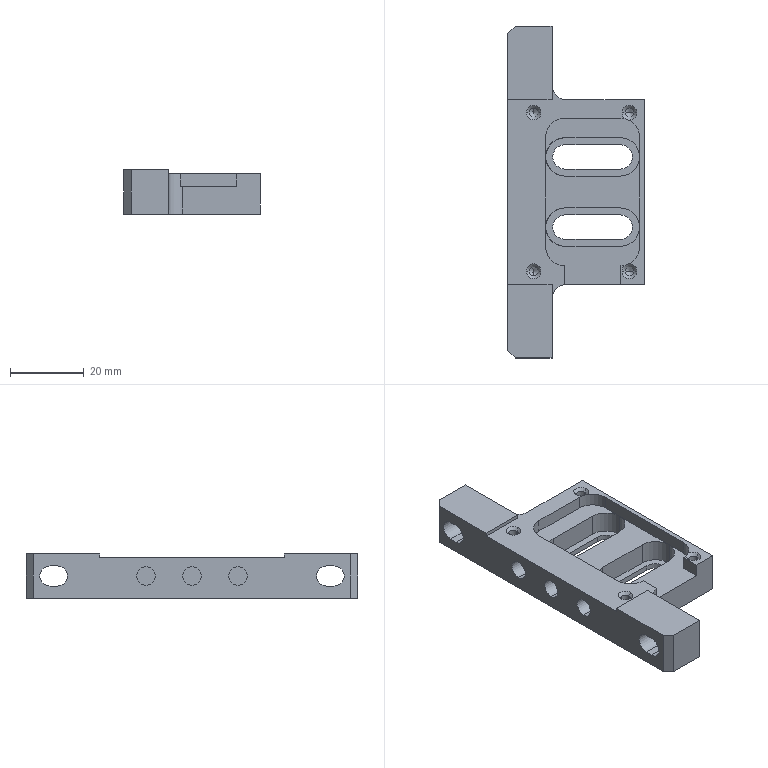Part | SolidWorks | features BaseBody 1 | 1 solid | 105 faces | box 37 x 90 x 12 mm | volume 17077 mm3 | plane 47 | cylinder 42 | cone 16 | commonest cylinder face diameters 10 x10 2.5 x8 5 x6 6.6 x6 10.4 x6 5.5 x4